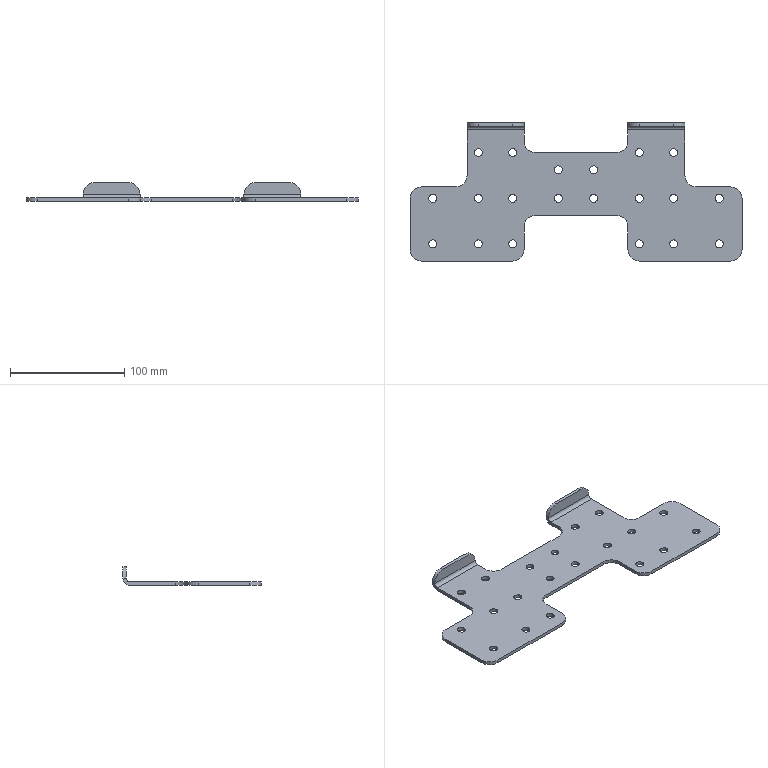Part | STEP file | Part5 | 1 solid | 62 faces | box 291 x 121 x 16.288 mm | volume 71655 mm3 | cylinder 40 | plane 22 | commonest cylinder face diameters 7 x20 20 x16 6 x2 12 x2